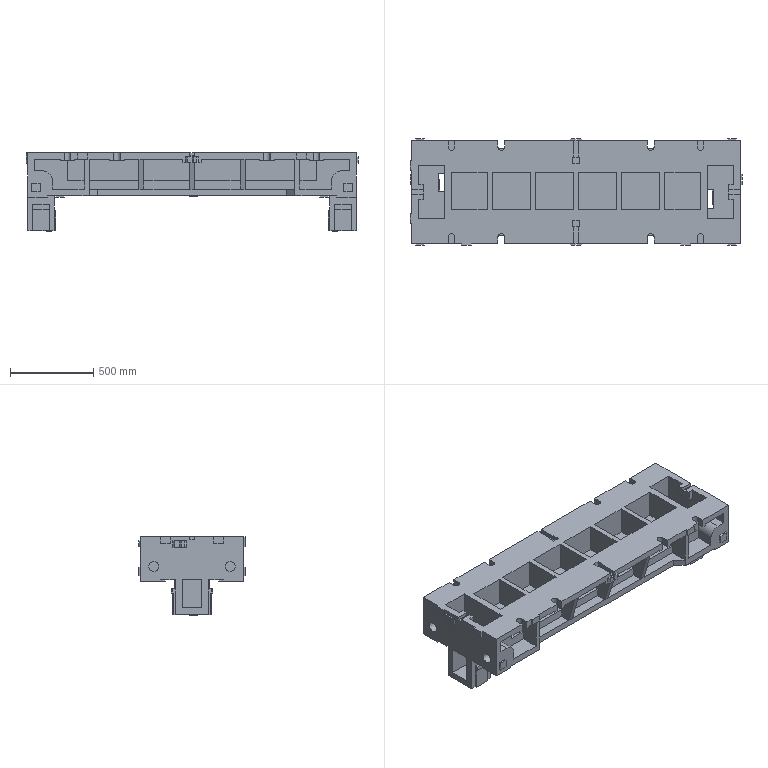Part | NX | features solid 2 | 1 solid | 580 faces | box 2000 x 640 x 475 mm | volume 146467854 mm3 | plane 546 | cylinder 34 | commonest cylinder face diameters 40 x8 90 x8 30 x6 60 x4 120 x4 10 x3